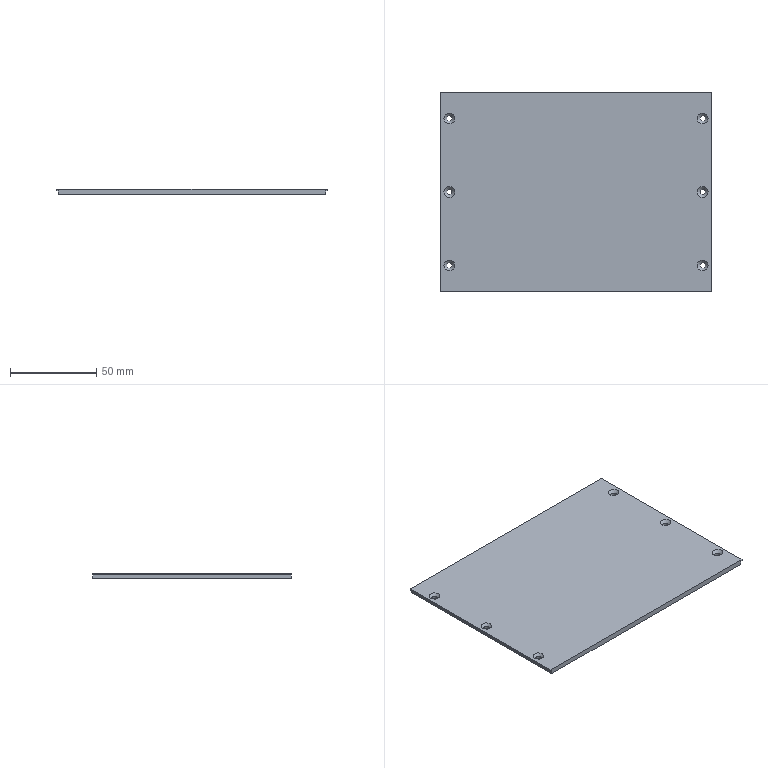CAM job | NX | 3-axis milling, drilling | part box 156.6 x 115 x 3 mm | stock box 156.6 x 115 x 3 mm
Tools:
number,name,description,diameter,corner_radius,flute_length,length,flutes
3,T3-D10-CX,Milling Tool-5 Parameters,10.0,0.0,50.0,75.0,2
4,T4-D10-JX,Milling Tool-5 Parameters,10.0,0.0,50.0,75.0,2
6,T6-D8-JX,Milling Tool-5 Parameters,8.0,0.0,50.0,75.0,2
10,T10-D4-90DEG,Drilling Tool,4.0,0.0,35.0,50.0,2
13,T13-ZT3.2,Drilling Tool,3.2,0.0,35.0,50.0,2
Operations:
program,operation,operation_type,tool,method,geometry_group,spindle_rpm,surface_speed,feed_per_tooth,feed_cut,feed_plunge,cut_length_mm,path_length_mm,cut_time_min,machine_time_min
A01,A1,PlanarMilling,T3-D10-CX,METHOD,WORKPIECE,6500.0,122.0,0.1154,1500.0,100.0,337.2,777.217,0.2248,0.2971
A01,A2,PlanarMilling,T4-D10-JX,METHOD,WORKPIECE,6500.0,122.0,0.1154,1500.0,100.0,337.2,776.217,0.2248,0.2969
A01,A3-M00,PlanarMilling,T10-D4-90DEG,METHOD,WORKPIECE,6500.0,122.0,0.1154,1500.0,100.0,324.0,745.018,0.216,0.285
A04,B1,PlanarMilling,T3-D10-CX,METHOD,WORKPIECE,6500.0,122.0,0.1154,1500.0,100.0,254.0,726.418,0.1693,0.2485
A04,B2,PlanarMilling,T3-D10-CX,METHOD,WORKPIECE,6500.0,122.0,0.1154,1500.0,100.0,254.0,735.217,0.1693,0.2499
A04,B2-1,CavityMilling,T3-D10-CX,METHOD,WORKPIECE,6500.0,122.0,0.1923,2500.0,100.0,2251.063,3265.151,0.9004,1.042
A04,B3,PlanarMilling,T4-D10-JX,METHOD,WORKPIECE,6500.0,122.0,0.1154,1500.0,100.0,254.0,727.018,0.1693,0.2485
A04,B4,PlanarMilling,T4-D10-JX,METHOD,WORKPIECE,6500.0,122.0,0.1154,1500.0,100.0,254.0,734.617,0.1693,0.2498
A04,B5,CavityMilling,T6-D8-JX,METHOD,WORKPIECE,6000.0,150.0,0.0833,1000.0,100.0,3209.873,4228.079,3.21,3.353
A04,B5_COPY,CavityMilling,T6-D8-JX,METHOD,WORKPIECE,6000.0,150.0,0.0833,1000.0,100.0,3209.873,4240.079,3.21,3.355
A04,B6,PlanarMilling,T10-D4-90DEG,METHOD,WORKPIECE,6500.0,122.0,0.1154,1500.0,100.0,931.57,2006.222,0.621,0.7689
A04,B7,PlanarMilling,T10-D4-90DEG,METHOD,WORKPIECE,6500.0,122.0,0.1154,1500.0,100.0,240.8,708.217,0.1605,0.2386
A04,B8,PlanarMilling,T10-D4-90DEG,METHOD,WORKPIECE,6500.0,122.0,0.1154,1500.0,100.0,240.8,701.418,0.1605,0.2375
A04,B9,Operation,T10-D4-90DEG,METHOD,WORKPIECE,1200.0,18.0,0.0417,100.0,0.0,18.9,462.014,0.189,0.2333
A04,B10,Operation,T13-ZT3.2,METHOD,WORKPIECE,1200.0,18.0,0.0417,100.0,0.0,45.0,514.213,0.45,0.4969